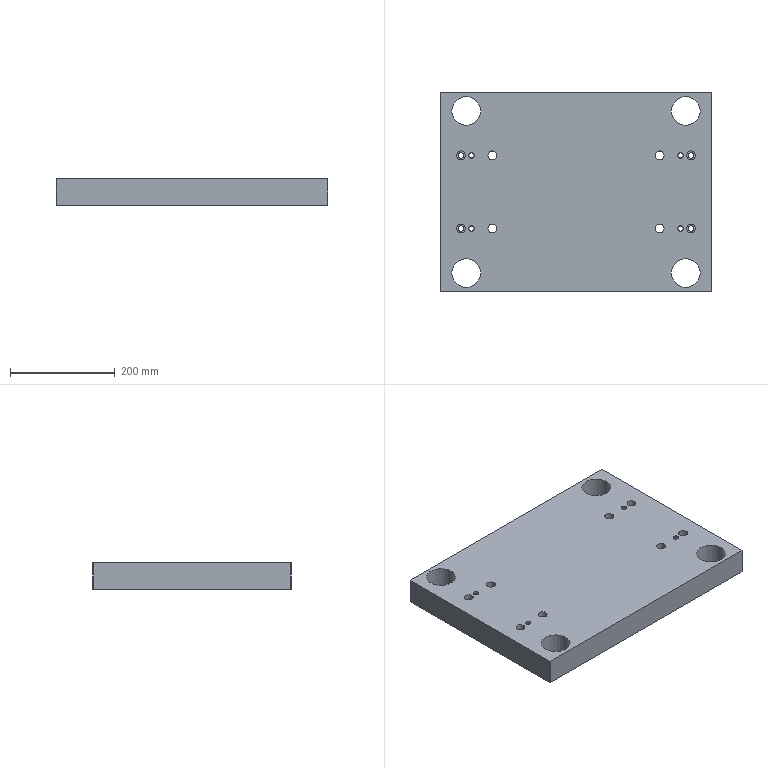Part | NX | features BREP 1 | 1 solid | 42 faces | box 520 x 380 x 50 mm | volume 9317025 mm3 | cylinder 24 | plane 18 | commonest cylinder face diameters 17 x8 10 x4 10.8 x4 11 x4 55 x4
STEP:
#1=CARTESIAN_POINT('',(-260.,-189.,117.));
#2=VERTEX_POINT('',#1);
#3=CARTESIAN_POINT('',(-260.,189.,117.));
#4=VERTEX_POINT('',#3);
#5=CARTESIAN_POINT('',(-260.,-190.,117.));
#6=DIRECTION('',(0.,1.,0.));
#7=VECTOR('',#6,1000.);
#8=LINE('',#5,#7);
#9=EDGE_CURVE('',#2,#4,#8,.T.);
#10=ORIENTED_EDGE('',*,*,#9,.T.);
#11=CARTESIAN_POINT('',(-260.,189.,67.));
#12=VERTEX_POINT('',#11);
#13=CARTESIAN_POINT('',(-260.,189.,67.));
#14=DIRECTION('',(0.,0.,-1.));
#15=VECTOR('',#14,1000.);
#16=LINE('',#13,#15);
#17=EDGE_CURVE('',#4,#12,#16,.T.);
#18=ORIENTED_EDGE('',*,*,#17,.T.);
#19=CARTESIAN_POINT('',(-260.,-189.,67.));
#20=VERTEX_POINT('',#19);
#21=CARTESIAN_POINT('',(-260.,-190.,67.));
#22=DIRECTION('',(0.,1.,0.));
#23=VECTOR('',#22,1000.);
#24=LINE('',#21,#23);
#25=EDGE_CURVE('',#20,#12,#24,.T.);
#26=ORIENTED_EDGE('',*,*,#25,.F.);
#27=CARTESIAN_POINT('',(-260.,-189.,67.));
#28=DIRECTION('',(0.,0.,1.));
#29=VECTOR('',#28,1000.);
#30=LINE('',#27,#29);
#31=EDGE_CURVE('',#20,#2,#30,.T.);
#32=ORIENTED_EDGE('',*,*,#31,.T.);
#33=EDGE_LOOP('',(#10,#18,#26,#32));
#34=FACE_BOUND('',#33,.T.);
#35=CARTESIAN_POINT('',(-260.,-190.,67.));
#36=DIRECTION('',(1.,0.,0.));
#37=DIRECTION('',(0.,0.,1.));
#38=AXIS2_PLACEMENT_3D('',#35,#36,#37);
#39=PLANE('',#38);
#40=ADVANCED_FACE('',(#34),#39,.F.);
#41=CARTESIAN_POINT('',(-259.,190.,67.));
#42=VERTEX_POINT('',#41);
#43=CARTESIAN_POINT('',(259.,190.,67.));
#44=VERTEX_POINT('',#43);
#45=CARTESIAN_POINT('',(-260.,190.,67.));
#46=DIRECTION('',(1.,0.,0.));
#47=VECTOR('',#46,1000.);
#48=LINE('',#45,#47);
#49=EDGE_CURVE('',#42,#44,#48,.T.);
#50=ORIENTED_EDGE('',*,*,#49,.F.);
#51=CARTESIAN_POINT('',(-259.,190.,117.));
#52=VERTEX_POINT('',#51);
#53=CARTESIAN_POINT('',(-259.,190.,67.));
#54=DIRECTION('',(0.,0.,1.));
#55=VECTOR('',#54,1000.);
#56=LINE('',#53,#55);
#57=EDGE_CURVE('',#42,#52,#56,.T.);
#58=ORIENTED_EDGE('',*,*,#57,.T.);
#59=CARTESIAN_POINT('',(259.,190.,117.));
#60=VERTEX_POINT('',#59);
#61=CARTESIAN_POINT('',(-260.,190.,117.));
#62=DIRECTION('',(1.,0.,0.));
#63=VECTOR('',#62,1000.);
#64=LINE('',#61,#63);
#65=EDGE_CURVE('',#52,#60,#64,.T.);
#66=ORIENTED_EDGE('',*,*,#65,.T.);
#67=CARTESIAN_POINT('',(259.,190.,67.));
#68=DIRECTION('',(0.,0.,-1.));
#69=VECTOR('',#68,1000.);
#70=LINE('',#67,#69);
#71=EDGE_CURVE('',#60,#44,#70,.T.);
#72=ORIENTED_EDGE('',*,*,#71,.T.);
#73=EDGE_LOOP('',(#50,#58,#66,#72));
#74=FACE_BOUND('',#73,.T.);
#75=CARTESIAN_POINT('',(-260.,190.,67.));
#76=DIRECTION('',(0.,-1.,0.));
#77=DIRECTION('',(0.,0.,1.));
#78=AXIS2_PLACEMENT_3D('',#75,#76,#77);
#79=PLANE('',#78);
#80=ADVANCED_FACE('',(#74),#79,.F.);
#81=CARTESIAN_POINT('',(260.,189.,67.));
#82=VERTEX_POINT('',#81);
#83=CARTESIAN_POINT('',(260.,-189.,67.));
#84=VERTEX_POINT('',#83);
#85=CARTESIAN_POINT('',(260.,190.,67.));
#86=DIRECTION('',(0.,-1.,0.));
#87=VECTOR('',#86,1000.);
#88=LINE('',#85,#87);
#89=EDGE_CURVE('',#82,#84,#88,.T.);
#90=ORIENTED_EDGE('',*,*,#89,.F.);
#91=CARTESIAN_POINT('',(260.,189.,117.));
#92=VERTEX_POINT('',#91);
#93=CARTESIAN_POINT('',(260.,189.,67.));
#94=DIRECTION('',(0.,0.,1.));
#95=VECTOR('',#94,1000.);
#96=LINE('',#93,#95);
#97=EDGE_CURVE('',#82,#92,#96,.T.);
#98=ORIENTED_EDGE('',*,*,#97,.T.);
#99=CARTESIAN_POINT('',(260.,-189.,117.));
#100=VERTEX_POINT('',#99);
#101=CARTESIAN_POINT('',(260.,190.,117.));
#102=DIRECTION('',(0.,-1.,0.));
#103=VECTOR('',#102,1000.);
#104=LINE('',#101,#103);
#105=EDGE_CURVE('',#92,#100,#104,.T.);
#106=ORIENTED_EDGE('',*,*,#105,.T.);
#107=CARTESIAN_POINT('',(260.,-189.,67.));
#108=DIRECTION('',(0.,0.,-1.));
#109=VECTOR('',#108,1000.);
#110=LINE('',#107,#109);
#111=EDGE_CURVE('',#100,#84,#110,.T.);
#112=ORIENTED_EDGE('',*,*,#111,.T.);
#113=EDGE_LOOP('',(#90,#98,#106,#112));
#114=FACE_BOUND('',#113,.T.);
#115=CARTESIAN_POINT('',(260.,190.,67.));
#116=DIRECTION('',(-1.,0.,0.));
#117=DIRECTION('',(0.,0.,-1.));
#118=AXIS2_PLACEMENT_3D('',#115,#116,#117);
#119=PLANE('',#118);
#120=ADVANCED_FACE('',(#114),#119,.F.);
#121=CARTESIAN_POINT('',(259.,-190.,67.));
#122=VERTEX_POINT('',#121);
#123=CARTESIAN_POINT('',(-259.,-190.,67.));
#124=VERTEX_POINT('',#123);
#125=CARTESIAN_POINT('',(260.,-190.,67.));
#126=DIRECTION('',(-1.,0.,0.));
#127=VECTOR('',#126,1000.);
#128=LINE('',#125,#127);
#129=EDGE_CURVE('',#122,#124,#128,.T.);
#130=ORIENTED_EDGE('',*,*,#129,.F.);
#131=CARTESIAN_POINT('',(259.,-190.,117.));
#132=VERTEX_POINT('',#131);
#133=CARTESIAN_POINT('',(259.,-190.,67.));
#134=DIRECTION('',(0.,0.,1.));
#135=VECTOR('',#134,1000.);
#136=LINE('',#133,#135);
#137=EDGE_CURVE('',#122,#132,#136,.T.);
#138=ORIENTED_EDGE('',*,*,#137,.T.);
#139=CARTESIAN_POINT('',(-259.,-190.,117.));
#140=VERTEX_POINT('',#139);
#141=CARTESIAN_POINT('',(260.,-190.,117.));
#142=DIRECTION('',(-1.,0.,0.));
#143=VECTOR('',#142,1000.);
#144=LINE('',#141,#143);
#145=EDGE_CURVE('',#132,#140,#144,.T.);
#146=ORIENTED_EDGE('',*,*,#145,.T.);
#147=CARTESIAN_POINT('',(-259.,-190.,67.));
#148=DIRECTION('',(0.,0.,-1.));
#149=VECTOR('',#148,1000.);
#150=LINE('',#147,#149);
#151=EDGE_CURVE('',#140,#124,#150,.T.);
#152=ORIENTED_EDGE('',*,*,#151,.T.);
#153=EDGE_LOOP('',(#130,#138,#146,#152));
#154=FACE_BOUND('',#153,.T.);
#155=CARTESIAN_POINT('',(260.,-190.,67.));
#156=DIRECTION('',(0.,1.,0.));
#157=DIRECTION('',(1.,0.,0.));
#158=AXIS2_PLACEMENT_3D('',#155,#156,#157);
#159=PLANE('',#158);
#160=ADVANCED_FACE('',(#154),#159,.F.);
#161=CARTESIAN_POINT('',(182.5,-155.,67.));
#162=VERTEX_POINT('',#161);
#163=CARTESIAN_POINT('',(210.,-155.,67.));
#164=DIRECTION('',(0.,0.,1.));
#165=DIRECTION('',(-1.,0.,0.));
#166=AXIS2_PLACEMENT_3D('',#163,#164,#165);
#167=CIRCLE('',#166,27.5);
#168=EDGE_CURVE('',#162,#162,#167,.T.);
#169=ORIENTED_EDGE('',*,*,#168,.T.);
#170=EDGE_LOOP('',(#169));
#171=FACE_BOUND('',#170,.T.);
#172=CARTESIAN_POINT('',(-237.5,-155.,67.));
#173=VERTEX_POINT('',#172);
#174=CARTESIAN_POINT('',(-210.,-155.,67.));
#175=DIRECTION('',(0.,0.,1.));
#176=DIRECTION('',(-1.,0.,0.));
#177=AXIS2_PLACEMENT_3D('',#174,#175,#176);
#178=CIRCLE('',#177,27.5);
#179=EDGE_CURVE('',#173,#173,#178,.T.);
#180=ORIENTED_EDGE('',*,*,#179,.T.);
#181=EDGE_LOOP('',(#180));
#182=FACE_BOUND('',#181,.T.);
#183=CARTESIAN_POINT('',(-237.5,155.,67.));
#184=VERTEX_POINT('',#183);
#185=CARTESIAN_POINT('',(-210.,155.,67.));
#186=DIRECTION('',(0.,0.,1.));
#187=DIRECTION('',(-1.,0.,0.));
#188=AXIS2_PLACEMENT_3D('',#185,#186,#187);
#189=CIRCLE('',#188,27.5);
#190=EDGE_CURVE('',#184,#184,#189,.T.);
#191=ORIENTED_EDGE('',*,*,#190,.T.);
#192=EDGE_LOOP('',(#191));
#193=FACE_BOUND('',#192,.T.);
#194=CARTESIAN_POINT('',(182.5,155.,67.));
#195=VERTEX_POINT('',#194);
#196=CARTESIAN_POINT('',(210.,155.,67.));
#197=DIRECTION('',(0.,0.,1.));
#198=DIRECTION('',(-1.,0.,0.));
#199=AXIS2_PLACEMENT_3D('',#196,#197,#198);
#200=CIRCLE('',#199,27.5);
#201=EDGE_CURVE('',#195,#195,#200,.T.);
#202=ORIENTED_EDGE('',*,*,#201,.T.);
#203=EDGE_LOOP('',(#202));
#204=FACE_BOUND('',#203,.T.);
#205=CARTESIAN_POINT('',(214.5,-70.,67.));
#206=VERTEX_POINT('',#205);
#207=CARTESIAN_POINT('',(220.,-70.,67.));
#208=DIRECTION('',(0.,0.,-1.));
#209=DIRECTION('',(-1.,0.,0.));
#210=AXIS2_PLACEMENT_3D('',#207,#208,#209);
#211=CIRCLE('',#210,5.5);
#212=EDGE_CURVE('',#206,#206,#211,.T.);
#213=ORIENTED_EDGE('',*,*,#212,.F.);
#214=EDGE_LOOP('',(#213));
#215=FACE_BOUND('',#214,.T.);
#216=CARTESIAN_POINT('',(-225.5,70.,67.));
#217=VERTEX_POINT('',#216);
#218=CARTESIAN_POINT('',(-220.,70.,67.));
#219=DIRECTION('',(0.,0.,-1.));
#220=DIRECTION('',(-1.,0.,0.));
#221=AXIS2_PLACEMENT_3D('',#218,#219,#220);
#222=CIRCLE('',#221,5.5);
#223=EDGE_CURVE('',#217,#217,#222,.T.);
#224=ORIENTED_EDGE('',*,*,#223,.F.);
#225=EDGE_LOOP('',(#224));
#226=FACE_BOUND('',#225,.T.);
#227=CARTESIAN_POINT('',(-225.5,-70.,67.));
#228=VERTEX_POINT('',#227);
#229=CARTESIAN_POINT('',(-220.,-70.,67.));
#230=DIRECTION('',(0.,0.,-1.));
#231=DIRECTION('',(-1.,0.,0.));
#232=AXIS2_PLACEMENT_3D('',#229,#230,#231);
#233=CIRCLE('',#232,5.5);
#234=EDGE_CURVE('',#228,#228,#233,.T.);
#235=ORIENTED_EDGE('',*,*,#234,.F.);
#236=EDGE_LOOP('',(#235));
#237=FACE_BOUND('',#236,.T.);
#238=CARTESIAN_POINT('',(214.5,70.,67.));
#239=VERTEX_POINT('',#238);
#240=CARTESIAN_POINT('',(220.,70.,67.));
#241=DIRECTION('',(0.,0.,-1.));
#242=DIRECTION('',(-1.,0.,0.));
#243=AXIS2_PLACEMENT_3D('',#240,#241,#242);
#244=CIRCLE('',#243,5.5);
#245=EDGE_CURVE('',#239,#239,#244,.T.);
#246=ORIENTED_EDGE('',*,*,#245,.F.);
#247=EDGE_LOOP('',(#246));
#248=FACE_BOUND('',#247,.T.);
#249=CARTESIAN_POINT('',(168.5,-70.,67.));
#250=VERTEX_POINT('',#249);
#251=CARTESIAN_POINT('',(160.,-70.,67.));
#252=DIRECTION('',(0.,0.,1.));
#253=DIRECTION('',(1.,0.,0.));
#254=AXIS2_PLACEMENT_3D('',#251,#252,#253);
#255=CIRCLE('',#254,8.5);
#256=EDGE_CURVE('',#250,#250,#255,.T.);
#257=ORIENTED_EDGE('',*,*,#256,.T.);
#258=EDGE_LOOP('',(#257));
#259=FACE_BOUND('',#258,.T.);
#260=CARTESIAN_POINT('',(-151.5,70.,67.));
#261=VERTEX_POINT('',#260);
#262=CARTESIAN_POINT('',(-160.,70.,67.));
#263=DIRECTION('',(0.,0.,1.));
#264=DIRECTION('',(1.,0.,0.));
#265=AXIS2_PLACEMENT_3D('',#262,#263,#264);
#266=CIRCLE('',#265,8.5);
#267=EDGE_CURVE('',#261,#261,#266,.T.);
#268=ORIENTED_EDGE('',*,*,#267,.T.);
#269=EDGE_LOOP('',(#268));
#270=FACE_BOUND('',#269,.T.);
#271=CARTESIAN_POINT('',(-151.5,-70.,67.));
#272=VERTEX_POINT('',#271);
#273=CARTESIAN_POINT('',(-160.,-70.,67.));
#274=DIRECTION('',(0.,0.,1.));
#275=DIRECTION('',(1.,0.,0.));
#276=AXIS2_PLACEMENT_3D('',#273,#274,#275);
#277=CIRCLE('',#276,8.5);
#278=EDGE_CURVE('',#272,#272,#277,.T.);
#279=ORIENTED_EDGE('',*,*,#278,.T.);
#280=EDGE_LOOP('',(#279));
#281=FACE_BOUND('',#280,.T.);
#282=CARTESIAN_POINT('',(168.5,70.,67.));
#283=VERTEX_POINT('',#282);
#284=CARTESIAN_POINT('',(160.,70.,67.));
#285=DIRECTION('',(0.,0.,1.));
#286=DIRECTION('',(1.,0.,0.));
#287=AXIS2_PLACEMENT_3D('',#284,#285,#286);
#288=CIRCLE('',#287,8.5);
#289=EDGE_CURVE('',#283,#283,#288,.T.);
#290=ORIENTED_EDGE('',*,*,#289,.T.);
#291=EDGE_LOOP('',(#290));
#292=FACE_BOUND('',#291,.T.);
#293=ORIENTED_EDGE('',*,*,#25,.T.);
#294=CARTESIAN_POINT('',(-259.5,189.5,67.));
#295=DIRECTION('',(0.7071,0.7071,0.));
#296=VECTOR('',#295,1000.);
#297=LINE('',#294,#296);
#298=EDGE_CURVE('',#12,#42,#297,.T.);
#299=ORIENTED_EDGE('',*,*,#298,.T.);
#300=ORIENTED_EDGE('',*,*,#49,.T.);
#301=CARTESIAN_POINT('',(-0.5,449.5,67.));
#302=DIRECTION('',(0.7071,-0.7071,0.));
#303=VECTOR('',#302,1000.);
#304=LINE('',#301,#303);
#305=EDGE_CURVE('',#44,#82,#304,.T.);
#306=ORIENTED_EDGE('',*,*,#305,.T.);
#307=ORIENTED_EDGE('',*,*,#89,.T.);
#308=CARTESIAN_POINT('',(189.5,-259.5,67.));
#309=DIRECTION('',(-0.7071,-0.7071,0.));
#310=VECTOR('',#309,1000.);
#311=LINE('',#308,#310);
#312=EDGE_CURVE('',#84,#122,#311,.T.);
#313=ORIENTED_EDGE('',*,*,#312,.T.);
#314=ORIENTED_EDGE('',*,*,#129,.T.);
#315=CARTESIAN_POINT('',(-449.5,0.5,67.));
#316=DIRECTION('',(-0.7071,0.7071,0.));
#317=VECTOR('',#316,1000.);
#318=LINE('',#315,#317);
#319=EDGE_CURVE('',#124,#20,#318,.T.);
#320=ORIENTED_EDGE('',*,*,#319,.T.);
#321=EDGE_LOOP('',(#293,#299,#300,#306,#307,#313,#314,#320));
#322=FACE_BOUND('',#321,.T.);
#323=CARTESIAN_POINT('',(-204.619,-68.085,67.));
#324=VERTEX_POINT('',#323);
#325=CARTESIAN_POINT('',(-200.,-70.,67.));
#326=DIRECTION('',(0.,0.,-1.));
#327=DIRECTION('',(-0.9237,0.383,0.));
#328=AXIS2_PLACEMENT_3D('',#325,#326,#327);
#329=CIRCLE('',#328,5.);
#330=EDGE_CURVE('',#324,#324,#329,.T.);
#331=ORIENTED_EDGE('',*,*,#330,.F.);
#332=EDGE_LOOP('',(#331));
#333=FACE_BOUND('',#332,.T.);
#334=CARTESIAN_POINT('',(-204.619,71.915,67.));
#335=VERTEX_POINT('',#334);
#336=CARTESIAN_POINT('',(-200.,70.,67.));
#337=DIRECTION('',(0.,0.,-1.));
#338=DIRECTION('',(-0.9237,0.383,0.));
#339=AXIS2_PLACEMENT_3D('',#336,#337,#338);
#340=CIRCLE('',#339,5.);
#341=EDGE_CURVE('',#335,#335,#340,.T.);
#342=ORIENTED_EDGE('',*,*,#341,.F.);
#343=EDGE_LOOP('',(#342));
#344=FACE_BOUND('',#343,.T.);
#345=CARTESIAN_POINT('',(195.381,-68.085,67.));
#346=VERTEX_POINT('',#345);
#347=CARTESIAN_POINT('',(200.,-70.,67.));
#348=DIRECTION('',(0.,0.,-1.));
#349=DIRECTION('',(-0.9237,0.383,0.));
#350=AXIS2_PLACEMENT_3D('',#347,#348,#349);
#351=CIRCLE('',#350,5.);
#352=EDGE_CURVE('',#346,#346,#351,.T.);
#353=ORIENTED_EDGE('',*,*,#352,.F.);
#354=EDGE_LOOP('',(#353));
#355=FACE_BOUND('',#354,.T.);
#356=CARTESIAN_POINT('',(195.381,71.915,67.));
#357=VERTEX_POINT('',#356);
#358=CARTESIAN_POINT('',(200.,70.,67.));
#359=DIRECTION('',(0.,0.,-1.));
#360=DIRECTION('',(-0.9237,0.383,0.));
#361=AXIS2_PLACEMENT_3D('',#358,#359,#360);
#362=CIRCLE('',#361,5.);
#363=EDGE_CURVE('',#357,#357,#362,.T.);
#364=ORIENTED_EDGE('',*,*,#363,.F.);
#365=EDGE_LOOP('',(#364));
#366=FACE_BOUND('',#365,.T.);
#367=CARTESIAN_POINT('',(-260.,190.,67.));
#368=DIRECTION('',(0.,0.,-1.));
#369=DIRECTION('',(1.,0.,0.));
#370=AXIS2_PLACEMENT_3D('',#367,#368,#369);
#371=PLANE('',#370);
#372=ADVANCED_FACE('',(#171,#182,#193,#204,#215,#226,#237,#248,#259,#270,#281,#292,#322,#333,#344,#355,#366),#371,.T.);
#373=CARTESIAN_POINT('',(182.5,-155.,117.));
#374=VERTEX_POINT('',#373);
#375=CARTESIAN_POINT('',(210.,-155.,117.));
#376=DIRECTION('',(0.,0.,1.));
#377=DIRECTION('',(-1.,0.,0.));
#378=AXIS2_PLACEMENT_3D('',#375,#376,#377);
#379=CIRCLE('',#378,27.5);
#380=EDGE_CURVE('',#374,#374,#379,.T.);
#381=ORIENTED_EDGE('',*,*,#380,.F.);
#382=EDGE_LOOP('',(#381));
#383=FACE_BOUND('',#382,.T.);
#384=CARTESIAN_POINT('',(-237.5,-155.,117.));
#385=VERTEX_POINT('',#384);
#386=CARTESIAN_POINT('',(-210.,-155.,117.));
#387=DIRECTION('',(0.,0.,1.));
#388=DIRECTION('',(-1.,0.,0.));
#389=AXIS2_PLACEMENT_3D('',#386,#387,#388);
#390=CIRCLE('',#389,27.5);
#391=EDGE_CURVE('',#385,#385,#390,.T.);
#392=ORIENTED_EDGE('',*,*,#391,.F.);
#393=EDGE_LOOP('',(#392));
#394=FACE_BOUND('',#393,.T.);
#395=CARTESIAN_POINT('',(-237.5,155.,117.));
#396=VERTEX_POINT('',#395);
#397=CARTESIAN_POINT('',(-210.,155.,117.));
#398=DIRECTION('',(0.,0.,1.));
#399=DIRECTION('',(-1.,0.,0.));
#400=AXIS2_PLACEMENT_3D('',#397,#398,#399);
#401=CIRCLE('',#400,27.5);
#402=EDGE_CURVE('',#396,#396,#401,.T.);
#403=ORIENTED_EDGE('',*,*,#402,.F.);
#404=EDGE_LOOP('',(#403));
#405=FACE_BOUND('',#404,.T.);
#406=CARTESIAN_POINT('',(182.5,155.,117.));
#407=VERTEX_POINT('',#406);
#408=CARTESIAN_POINT('',(210.,155.,117.));
#409=DIRECTION('',(0.,0.,1.));
#410=DIRECTION('',(-1.,0.,0.));
#411=AXIS2_PLACEMENT_3D('',#408,#409,#410);
#412=CIRCLE('',#411,27.5);
#413=EDGE_CURVE('',#407,#407,#412,.T.);
#414=ORIENTED_EDGE('',*,*,#413,.F.);
#415=EDGE_LOOP('',(#414));
#416=FACE_BOUND('',#415,.T.);
#417=CARTESIAN_POINT('',(204.988,67.932,117.));
#418=VERTEX_POINT('',#417);
#419=CARTESIAN_POINT('',(200.,70.,117.));
#420=DIRECTION('',(0.,0.,1.));
#421=DIRECTION('',(0.9237,-0.383,0.));
#422=AXIS2_PLACEMENT_3D('',#419,#420,#421);
#423=CIRCLE('',#422,5.4);
#424=EDGE_CURVE('',#418,#418,#423,.T.);
#425=ORIENTED_EDGE('',*,*,#424,.F.);
#426=EDGE_LOOP('',(#425));
#427=FACE_BOUND('',#426,.T.);
#428=CARTESIAN_POINT('',(204.988,-72.068,117.));
#429=VERTEX_POINT('',#428);
#430=CARTESIAN_POINT('',(200.,-70.,117.));
#431=DIRECTION('',(0.,0.,1.));
#432=DIRECTION('',(0.9237,-0.383,0.));
#433=AXIS2_PLACEMENT_3D('',#430,#431,#432);
#434=CIRCLE('',#433,5.4);
#435=EDGE_CURVE('',#429,#429,#434,.T.);
#436=ORIENTED_EDGE('',*,*,#435,.F.);
#437=EDGE_LOOP('',(#436));
#438=FACE_BOUND('',#437,.T.);
#439=CARTESIAN_POINT('',(-195.012,67.932,117.));
#440=VERTEX_POINT('',#439);
#441=CARTESIAN_POINT('',(-200.,70.,117.));
#442=DIRECTION('',(0.,0.,1.));
#443=DIRECTION('',(0.9237,-0.383,0.));
#444=AXIS2_PLACEMENT_3D('',#441,#442,#443);
#445=CIRCLE('',#444,5.4);
#446=EDGE_CURVE('',#440,#440,#445,.T.);
#447=ORIENTED_EDGE('',*,*,#446,.F.);
#448=EDGE_LOOP('',(#447));
#449=FACE_BOUND('',#448,.T.);
#450=CARTESIAN_POINT('',(-195.012,-72.068,117.));
#451=VERTEX_POINT('',#450);
#452=CARTESIAN_POINT('',(-200.,-70.,117.));
#453=DIRECTION('',(0.,0.,1.));
#454=DIRECTION('',(0.9237,-0.383,0.));
#455=AXIS2_PLACEMENT_3D('',#452,#453,#454);
#456=CIRCLE('',#455,5.4);
#457=EDGE_CURVE('',#451,#451,#456,.T.);
#458=ORIENTED_EDGE('',*,*,#457,.F.);
#459=EDGE_LOOP('',(#458));
#460=FACE_BOUND('',#459,.T.);
#461=CARTESIAN_POINT('',(228.5,-70.,117.));
#462=VERTEX_POINT('',#461);
#463=CARTESIAN_POINT('',(220.,-70.,117.));
#464=DIRECTION('',(0.,0.,1.));
#465=DIRECTION('',(1.,0.,0.));
#466=AXIS2_PLACEMENT_3D('',#463,#464,#465);
#467=CIRCLE('',#466,8.5);
#468=EDGE_CURVE('',#462,#462,#467,.T.);
#469=ORIENTED_EDGE('',*,*,#468,.F.);
#470=EDGE_LOOP('',(#469));
#471=FACE_BOUND('',#470,.T.);
#472=CARTESIAN_POINT('',(-211.5,70.,117.));
#473=VERTEX_POINT('',#472);
#474=CARTESIAN_POINT('',(-220.,70.,117.));
#475=DIRECTION('',(0.,0.,1.));
#476=DIRECTION('',(1.,0.,0.));
#477=AXIS2_PLACEMENT_3D('',#474,#475,#476);
#478=CIRCLE('',#477,8.5);
#479=EDGE_CURVE('',#473,#473,#478,.T.);
#480=ORIENTED_EDGE('',*,*,#479,.F.);
#481=EDGE_LOOP('',(#480));
#482=FACE_BOUND('',#481,.T.);
#483=CARTESIAN_POINT('',(-211.5,-70.,117.));
#484=VERTEX_POINT('',#483);
#485=CARTESIAN_POINT('',(-220.,-70.,117.));
#486=DIRECTION('',(0.,0.,1.));
#487=DIRECTION('',(1.,0.,0.));
#488=AXIS2_PLACEMENT_3D('',#485,#486,#487);
#489=CIRCLE('',#488,8.5);
#490=EDGE_CURVE('',#484,#484,#489,.T.);
#491=ORIENTED_EDGE('',*,*,#490,.F.);
#492=EDGE_LOOP('',(#491));
#493=FACE_BOUND('',#492,.T.);
#494=CARTESIAN_POINT('',(228.5,70.,117.));
#495=VERTEX_POINT('',#494);
#496=CARTESIAN_POINT('',(220.,70.,117.));
#497=DIRECTION('',(0.,0.,1.));
#498=DIRECTION('',(1.,0.,0.));
#499=AXIS2_PLACEMENT_3D('',#496,#497,#498);
#500=CIRCLE('',#499,8.5);
#501=EDGE_CURVE('',#495,#495,#500,.T.);
#502=ORIENTED_EDGE('',*,*,#501,.F.);
#503=EDGE_LOOP('',(#502));
#504=FACE_BOUND('',#503,.T.);
#505=CARTESIAN_POINT('',(168.5,-70.,117.));
#506=VERTEX_POINT('',#505);
#507=CARTESIAN_POINT('',(160.,-70.,117.));
#508=DIRECTION('',(0.,0.,1.));
#509=DIRECTION('',(1.,0.,0.));
#510=AXIS2_PLACEMENT_3D('',#507,#508,#509);
#511=CIRCLE('',#510,8.5);
#512=EDGE_CURVE('',#506,#506,#511,.T.);
#513=ORIENTED_EDGE('',*,*,#512,.F.);
#514=EDGE_LOOP('',(#513));
#515=FACE_BOUND('',#514,.T.);
#516=CARTESIAN_POINT('',(-151.5,70.,117.));
#517=VERTEX_POINT('',#516);
#518=CARTESIAN_POINT('',(-160.,70.,117.));
#519=DIRECTION('',(0.,0.,1.));
#520=DIRECTION('',(1.,0.,0.));
#521=AXIS2_PLACEMENT_3D('',#518,#519,#520);
#522=CIRCLE('',#521,8.5);
#523=EDGE_CURVE('',#517,#517,#522,.T.);
#524=ORIENTED_EDGE('',*,*,#523,.F.);
#525=EDGE_LOOP('',(#524));
#526=FACE_BOUND('',#525,.T.);
#527=CARTESIAN_POINT('',(-151.5,-70.,117.));
#528=VERTEX_POINT('',#527);
#529=CARTESIAN_POINT('',(-160.,-70.,117.));
#530=DIRECTION('',(0.,0.,1.));
#531=DIRECTION('',(1.,0.,0.));
#532=AXIS2_PLACEMENT_3D('',#529,#530,#531);
#533=CIRCLE('',#532,8.5);
#534=EDGE_CURVE('',#528,#528,#533,.T.);
#535=ORIENTED_EDGE('',*,*,#534,.F.);
#536=EDGE_LOOP('',(#535));
#537=FACE_BOUND('',#536,.T.);
#538=CARTESIAN_POINT('',(168.5,70.,117.));
#539=VERTEX_POINT('',#538);
#540=CARTESIAN_POINT('',(160.,70.,117.));
#541=DIRECTION('',(0.,0.,1.));
#542=DIRECTION('',(1.,0.,0.));
#543=AXIS2_PLACEMENT_3D('',#540,#541,#542);
#544=CIRCLE('',#543,8.5);
#545=EDGE_CURVE('',#539,#539,#544,.T.);
#546=ORIENTED_EDGE('',*,*,#545,.F.);
#547=EDGE_LOOP('',(#546));
#548=FACE_BOUND('',#547,.T.);
#549=ORIENTED_EDGE('',*,*,#65,.F.);
#550=CARTESIAN_POINT('',(-259.,190.,117.));
#551=DIRECTION('',(-0.7071,-0.7071,0.));
#552=VECTOR('',#551,1000.);
#553=LINE('',#550,#552);
#554=EDGE_CURVE('',#52,#4,#553,.T.);
#555=ORIENTED_EDGE('',*,*,#554,.T.);
#556=ORIENTED_EDGE('',*,*,#9,.F.);
#557=CARTESIAN_POINT('',(-260.,-189.,117.));
#558=DIRECTION('',(0.7071,-0.7071,0.));
#559=VECTOR('',#558,1000.);
#560=LINE('',#557,#559);
#561=EDGE_CURVE('',#2,#140,#560,.T.);
#562=ORIENTED_EDGE('',*,*,#561,.T.);
#563=ORIENTED_EDGE('',*,*,#145,.F.);
#564=CARTESIAN_POINT('',(259.,-190.,117.));
#565=DIRECTION('',(0.7071,0.7071,0.));
#566=VECTOR('',#565,1000.);
#567=LINE('',#564,#566);
#568=EDGE_CURVE('',#132,#100,#567,.T.);
#569=ORIENTED_EDGE('',*,*,#568,.T.);
#570=ORIENTED_EDGE('',*,*,#105,.F.);
#571=CARTESIAN_POINT('',(260.,189.,117.));
#572=DIRECTION('',(-0.7071,0.7071,0.));
#573=VECTOR('',#572,1000.);
#574=LINE('',#571,#573);
#575=EDGE_CURVE('',#92,#60,#574,.T.);
#576=ORIENTED_EDGE('',*,*,#575,.T.);
#577=EDGE_LOOP('',(#549,#555,#556,#562,#563,#569,#570,#576));
#578=FACE_BOUND('',#577,.T.);
#579=CARTESIAN_POINT('',(-260.,190.,117.));
#580=DIRECTION('',(0.,0.,-1.));
#581=DIRECTION('',(1.,0.,0.));
#582=AXIS2_PLACEMENT_3D('',#579,#580,#581);
#583=PLANE('',#582);
#584=ADVANCED_FACE('',(#383,#394,#405,#416,#427,#438,#449,#460,#471,#482,#493,#504,#515,#526,#537,#548,#578),#583,.F.);
#585=ORIENTED_EDGE('',*,*,#298,.F.);
#586=ORIENTED_EDGE('',*,*,#17,.F.);
#587=ORIENTED_EDGE('',*,*,#554,.F.);
#588=ORIENTED_EDGE('',*,*,#57,.F.);
#589=EDGE_LOOP('',(#585,#586,#587,#588));
#590=FACE_BOUND('',#589,.T.);
#591=CARTESIAN_POINT('',(-259.,190.,67.));
#592=DIRECTION('',(0.7071,-0.7071,0.));
#593=DIRECTION('',(-0.7071,-0.7071,0.));
#594=AXIS2_PLACEMENT_3D('',#591,#592,#593);
#595=PLANE('',#594);
#596=ADVANCED_FACE('',(#590),#595,.F.);
#597=ORIENTED_EDGE('',*,*,#305,.F.);
#598=ORIENTED_EDGE('',*,*,#71,.F.);
#599=ORIENTED_EDGE('',*,*,#575,.F.);
#600=ORIENTED_EDGE('',*,*,#97,.F.);
#601=EDGE_LOOP('',(#597,#598,#599,#600));
#602=FACE_BOUND('',#601,.T.);
#603=CARTESIAN_POINT('',(260.,189.,67.));
#604=DIRECTION('',(-0.7071,-0.7071,0.));
#605=DIRECTION('',(-0.7071,0.7071,0.));
#606=AXIS2_PLACEMENT_3D('',#603,#604,#605);
#607=PLANE('',#606);
#608=ADVANCED_FACE('',(#602),#607,.F.);
#609=ORIENTED_EDGE('',*,*,#312,.F.);
#610=ORIENTED_EDGE('',*,*,#111,.F.);
#611=ORIENTED_EDGE('',*,*,#568,.F.);
#612=ORIENTED_EDGE('',*,*,#137,.F.);
#613=EDGE_LOOP('',(#609,#610,#611,#612));
#614=FACE_BOUND('',#613,.T.);
#615=CARTESIAN_POINT('',(259.,-190.,67.));
#616=DIRECTION('',(-0.7071,0.7071,0.));
#617=DIRECTION('',(0.7071,0.7071,0.));
#618=AXIS2_PLACEMENT_3D('',#615,#616,#617);
#619=PLANE('',#618);
#620=ADVANCED_FACE('',(#614),#619,.F.);
#621=ORIENTED_EDGE('',*,*,#319,.F.);
#622=ORIENTED_EDGE('',*,*,#151,.F.);
#623=ORIENTED_EDGE('',*,*,#561,.F.);
#624=ORIENTED_EDGE('',*,*,#31,.F.);
#625=EDGE_LOOP('',(#621,#622,#623,#624));
#626=FACE_BOUND('',#625,.T.);
#627=CARTESIAN_POINT('',(-260.,-189.,67.));
#628=DIRECTION('',(0.7071,0.7071,0.));
#629=DIRECTION('',(0.7071,-0.7071,0.));
#630=AXIS2_PLACEMENT_3D('',#627,#628,#629);
#631=PLANE('',#630);
#632=ADVANCED_FACE('',(#626),#631,.F.);
#633=ORIENTED_EDGE('',*,*,#545,.T.);
#634=EDGE_LOOP('',(#633));
#635=FACE_BOUND('',#634,.T.);
#636=ORIENTED_EDGE('',*,*,#289,.F.);
#637=EDGE_LOOP('',(#636));
#638=FACE_BOUND('',#637,.T.);
#639=CARTESIAN_POINT('',(160.,70.,117.));
#640=DIRECTION('',(0.,0.,-1.));
#641=DIRECTION('',(1.,0.,0.));
#642=AXIS2_PLACEMENT_3D('',#639,#640,#641);
#643=CYLINDRICAL_SURFACE('',#642,8.5);
#644=ADVANCED_FACE('',(#635,#638),#643,.F.);
#645=ORIENTED_EDGE('',*,*,#534,.T.);
#646=EDGE_LOOP('',(#645));
#647=FACE_BOUND('',#646,.T.);
#648=ORIENTED_EDGE('',*,*,#278,.F.);
#649=EDGE_LOOP('',(#648));
#650=FACE_BOUND('',#649,.T.);
#651=CARTESIAN_POINT('',(-160.,-70.,117.));
#652=DIRECTION('',(0.,0.,-1.));
#653=DIRECTION('',(1.,0.,0.));
#654=AXIS2_PLACEMENT_3D('',#651,#652,#653);
#655=CYLINDRICAL_SURFACE('',#654,8.5);
#656=ADVANCED_FACE('',(#647,#650),#655,.F.);
#657=ORIENTED_EDGE('',*,*,#523,.T.);
#658=EDGE_LOOP('',(#657));
#659=FACE_BOUND('',#658,.T.);
#660=ORIENTED_EDGE('',*,*,#267,.F.);
#661=EDGE_LOOP('',(#660));
#662=FACE_BOUND('',#661,.T.);
#663=CARTESIAN_POINT('',(-160.,70.,117.));
#664=DIRECTION('',(0.,0.,-1.));
#665=DIRECTION('',(1.,0.,0.));
#666=AXIS2_PLACEMENT_3D('',#663,#664,#665);
#667=CYLINDRICAL_SURFACE('',#666,8.5);
#668=ADVANCED_FACE('',(#659,#662),#667,.F.);
#669=ORIENTED_EDGE('',*,*,#512,.T.);
#670=EDGE_LOOP('',(#669));
#671=FACE_BOUND('',#670,.T.);
#672=ORIENTED_EDGE('',*,*,#256,.F.);
#673=EDGE_LOOP('',(#672));
#674=FACE_BOUND('',#673,.T.);
#675=CARTESIAN_POINT('',(160.,-70.,117.));
#676=DIRECTION('',(0.,0.,-1.));
#677=DIRECTION('',(1.,0.,0.));
#678=AXIS2_PLACEMENT_3D('',#675,#676,#677);
#679=CYLINDRICAL_SURFACE('',#678,8.5);
#680=ADVANCED_FACE('',(#671,#674),#679,.F.);
#681=ORIENTED_EDGE('',*,*,#245,.T.);
#682=EDGE_LOOP('',(#681));
#683=FACE_BOUND('',#682,.T.);
#684=CARTESIAN_POINT('',(214.5,70.,103.));
#685=VERTEX_POINT('',#684);
#686=CARTESIAN_POINT('',(220.,70.,103.));
#687=DIRECTION('',(0.,0.,1.));
#688=DIRECTION('',(-1.,0.,0.));
#689=AXIS2_PLACEMENT_3D('',#686,#687,#688);
#690=CIRCLE('',#689,5.5);
#691=EDGE_CURVE('',#685,#685,#690,.T.);
#692=ORIENTED_EDGE('',*,*,#691,.T.);
#693=EDGE_LOOP('',(#692));
#694=FACE_BOUND('',#693,.T.);
#695=CARTESIAN_POINT('',(220.,70.,103.));
#696=DIRECTION('',(0.,0.,-1.));
#697=DIRECTION('',(1.,0.,0.));
#698=AXIS2_PLACEMENT_3D('',#695,#696,#697);
#699=CYLINDRICAL_SURFACE('',#698,5.5);
#700=ADVANCED_FACE('',(#683,#694),#699,.F.);
#701=ORIENTED_EDGE('',*,*,#501,.T.);
#702=EDGE_LOOP('',(#701));
#703=FACE_BOUND('',#702,.T.);
#704=CARTESIAN_POINT('',(228.5,70.,103.));
#705=VERTEX_POINT('',#704);
#706=CARTESIAN_POINT('',(220.,70.,103.));
#707=DIRECTION('',(0.,0.,-1.));
#708=DIRECTION('',(1.,0.,0.));
#709=AXIS2_PLACEMENT_3D('',#706,#707,#708);
#710=CIRCLE('',#709,8.5);
#711=EDGE_CURVE('',#705,#705,#710,.T.);
#712=ORIENTED_EDGE('',*,*,#711,.T.);
#713=EDGE_LOOP('',(#712));
#714=FACE_BOUND('',#713,.T.);
#715=CARTESIAN_POINT('',(220.,70.,103.));
#716=DIRECTION('',(0.,0.,1.));
#717=DIRECTION('',(-1.,0.,0.));
#718=AXIS2_PLACEMENT_3D('',#715,#716,#717);
#719=CYLINDRICAL_SURFACE('',#718,8.5);
#720=ADVANCED_FACE('',(#703,#714),#719,.F.);
#721=ORIENTED_EDGE('',*,*,#691,.F.);
#722=EDGE_LOOP('',(#721));
#723=FACE_BOUND('',#722,.T.);
#724=ORIENTED_EDGE('',*,*,#711,.F.);
#725=EDGE_LOOP('',(#724));
#726=FACE_BOUND('',#725,.T.);
#727=CARTESIAN_POINT('',(220.,70.,103.));
#728=DIRECTION('',(0.,0.,-1.));
#729=DIRECTION('',(1.,0.,0.));
#730=AXIS2_PLACEMENT_3D('',#727,#728,#729);
#731=PLANE('',#730);
#732=ADVANCED_FACE('',(#723,#726),#731,.F.);
#733=ORIENTED_EDGE('',*,*,#234,.T.);
#734=EDGE_LOOP('',(#733));
#735=FACE_BOUND('',#734,.T.);
#736=CARTESIAN_POINT('',(-225.5,-70.,103.));
#737=VERTEX_POINT('',#736);
#738=CARTESIAN_POINT('',(-220.,-70.,103.));
#739=DIRECTION('',(0.,0.,1.));
#740=DIRECTION('',(-1.,0.,0.));
#741=AXIS2_PLACEMENT_3D('',#738,#739,#740);
#742=CIRCLE('',#741,5.5);
#743=EDGE_CURVE('',#737,#737,#742,.T.);
#744=ORIENTED_EDGE('',*,*,#743,.T.);
#745=EDGE_LOOP('',(#744));
#746=FACE_BOUND('',#745,.T.);
#747=CARTESIAN_POINT('',(-220.,-70.,103.));
#748=DIRECTION('',(0.,0.,-1.));
#749=DIRECTION('',(1.,0.,0.));
#750=AXIS2_PLACEMENT_3D('',#747,#748,#749);
#751=CYLINDRICAL_SURFACE('',#750,5.5);
#752=ADVANCED_FACE('',(#735,#746),#751,.F.);
#753=ORIENTED_EDGE('',*,*,#490,.T.);
#754=EDGE_LOOP('',(#753));
#755=FACE_BOUND('',#754,.T.);
#756=CARTESIAN_POINT('',(-211.5,-70.,103.));
#757=VERTEX_POINT('',#756);
#758=CARTESIAN_POINT('',(-220.,-70.,103.));
#759=DIRECTION('',(0.,0.,-1.));
#760=DIRECTION('',(1.,0.,0.));
#761=AXIS2_PLACEMENT_3D('',#758,#759,#760);
#762=CIRCLE('',#761,8.5);
#763=EDGE_CURVE('',#757,#757,#762,.T.);
#764=ORIENTED_EDGE('',*,*,#763,.T.);
#765=EDGE_LOOP('',(#764));
#766=FACE_BOUND('',#765,.T.);
#767=CARTESIAN_POINT('',(-220.,-70.,103.));
#768=DIRECTION('',(0.,0.,1.));
#769=DIRECTION('',(-1.,0.,0.));
#770=AXIS2_PLACEMENT_3D('',#767,#768,#769);
#771=CYLINDRICAL_SURFACE('',#770,8.5);
#772=ADVANCED_FACE('',(#755,#766),#771,.F.);
#773=ORIENTED_EDGE('',*,*,#743,.F.);
#774=EDGE_LOOP('',(#773));
#775=FACE_BOUND('',#774,.T.);
#776=ORIENTED_EDGE('',*,*,#763,.F.);
#777=EDGE_LOOP('',(#776));
#778=FACE_BOUND('',#777,.T.);
#779=CARTESIAN_POINT('',(-220.,-70.,103.));
#780=DIRECTION('',(0.,0.,-1.));
#781=DIRECTION('',(1.,0.,0.));
#782=AXIS2_PLACEMENT_3D('',#779,#780,#781);
#783=PLANE('',#782);
#784=ADVANCED_FACE('',(#775,#778),#783,.F.);
#785=ORIENTED_EDGE('',*,*,#223,.T.);
#786=EDGE_LOOP('',(#785));
#787=FACE_BOUND('',#786,.T.);
#788=CARTESIAN_POINT('',(-225.5,70.,103.));
#789=VERTEX_POINT('',#788);
#790=CARTESIAN_POINT('',(-220.,70.,103.));
#791=DIRECTION('',(0.,0.,1.));
#792=DIRECTION('',(-1.,0.,0.));
#793=AXIS2_PLACEMENT_3D('',#790,#791,#792);
#794=CIRCLE('',#793,5.5);
#795=EDGE_CURVE('',#789,#789,#794,.T.);
#796=ORIENTED_EDGE('',*,*,#795,.T.);
#797=EDGE_LOOP('',(#796));
#798=FACE_BOUND('',#797,.T.);
#799=CARTESIAN_POINT('',(-220.,70.,103.));
#800=DIRECTION('',(0.,0.,-1.));
#801=DIRECTION('',(1.,0.,0.));
#802=AXIS2_PLACEMENT_3D('',#799,#800,#801);
#803=CYLINDRICAL_SURFACE('',#802,5.5);
#804=ADVANCED_FACE('',(#787,#798),#803,.F.);
#805=ORIENTED_EDGE('',*,*,#479,.T.);
#806=EDGE_LOOP('',(#805));
#807=FACE_BOUND('',#806,.T.);
#808=CARTESIAN_POINT('',(-211.5,70.,103.));
#809=VERTEX_POINT('',#808);
#810=CARTESIAN_POINT('',(-220.,70.,103.));
#811=DIRECTION('',(0.,0.,-1.));
#812=DIRECTION('',(1.,0.,0.));
#813=AXIS2_PLACEMENT_3D('',#810,#811,#812);
#814=CIRCLE('',#813,8.5);
#815=EDGE_CURVE('',#809,#809,#814,.T.);
#816=ORIENTED_EDGE('',*,*,#815,.T.);
#817=EDGE_LOOP('',(#816));
#818=FACE_BOUND('',#817,.T.);
#819=CARTESIAN_POINT('',(-220.,70.,103.));
#820=DIRECTION('',(0.,0.,1.));
#821=DIRECTION('',(-1.,0.,0.));
#822=AXIS2_PLACEMENT_3D('',#819,#820,#821);
#823=CYLINDRICAL_SURFACE('',#822,8.5);
#824=ADVANCED_FACE('',(#807,#818),#823,.F.);
#825=ORIENTED_EDGE('',*,*,#795,.F.);
#826=EDGE_LOOP('',(#825));
#827=FACE_BOUND('',#826,.T.);
#828=ORIENTED_EDGE('',*,*,#815,.F.);
#829=EDGE_LOOP('',(#828));
#830=FACE_BOUND('',#829,.T.);
#831=CARTESIAN_POINT('',(-220.,70.,103.));
#832=DIRECTION('',(0.,0.,-1.));
#833=DIRECTION('',(1.,0.,0.));
#834=AXIS2_PLACEMENT_3D('',#831,#832,#833);
#835=PLANE('',#834);
#836=ADVANCED_FACE('',(#827,#830),#835,.F.);
#837=ORIENTED_EDGE('',*,*,#212,.T.);
#838=EDGE_LOOP('',(#837));
#839=FACE_BOUND('',#838,.T.);
#840=CARTESIAN_POINT('',(214.5,-70.,103.));
#841=VERTEX_POINT('',#840);
#842=CARTESIAN_POINT('',(220.,-70.,103.));
#843=DIRECTION('',(0.,0.,1.));
#844=DIRECTION('',(-1.,0.,0.));
#845=AXIS2_PLACEMENT_3D('',#842,#843,#844);
#846=CIRCLE('',#845,5.5);
#847=EDGE_CURVE('',#841,#841,#846,.T.);
#848=ORIENTED_EDGE('',*,*,#847,.T.);
#849=EDGE_LOOP('',(#848));
#850=FACE_BOUND('',#849,.T.);
#851=CARTESIAN_POINT('',(220.,-70.,103.));
#852=DIRECTION('',(0.,0.,-1.));
#853=DIRECTION('',(1.,0.,0.));
#854=AXIS2_PLACEMENT_3D('',#851,#852,#853);
#855=CYLINDRICAL_SURFACE('',#854,5.5);
#856=ADVANCED_FACE('',(#839,#850),#855,.F.);
#857=ORIENTED_EDGE('',*,*,#468,.T.);
#858=EDGE_LOOP('',(#857));
#859=FACE_BOUND('',#858,.T.);
#860=CARTESIAN_POINT('',(228.5,-70.,103.));
#861=VERTEX_POINT('',#860);
#862=CARTESIAN_POINT('',(220.,-70.,103.));
#863=DIRECTION('',(0.,0.,-1.));
#864=DIRECTION('',(1.,0.,0.));
#865=AXIS2_PLACEMENT_3D('',#862,#863,#864);
#866=CIRCLE('',#865,8.5);
#867=EDGE_CURVE('',#861,#861,#866,.T.);
#868=ORIENTED_EDGE('',*,*,#867,.T.);
#869=EDGE_LOOP('',(#868));
#870=FACE_BOUND('',#869,.T.);
#871=CARTESIAN_POINT('',(220.,-70.,103.));
#872=DIRECTION('',(0.,0.,1.));
#873=DIRECTION('',(-1.,0.,0.));
#874=AXIS2_PLACEMENT_3D('',#871,#872,#873);
#875=CYLINDRICAL_SURFACE('',#874,8.5);
#876=ADVANCED_FACE('',(#859,#870),#875,.F.);
#877=ORIENTED_EDGE('',*,*,#847,.F.);
#878=EDGE_LOOP('',(#877));
#879=FACE_BOUND('',#878,.T.);
#880=ORIENTED_EDGE('',*,*,#867,.F.);
#881=EDGE_LOOP('',(#880));
#882=FACE_BOUND('',#881,.T.);
#883=CARTESIAN_POINT('',(220.,-70.,103.));
#884=DIRECTION('',(0.,0.,-1.));
#885=DIRECTION('',(1.,0.,0.));
#886=AXIS2_PLACEMENT_3D('',#883,#884,#885);
#887=PLANE('',#886);
#888=ADVANCED_FACE('',(#879,#882),#887,.F.);
#889=CARTESIAN_POINT('',(-195.012,-72.068,113.));
#890=VERTEX_POINT('',#889);
#891=CARTESIAN_POINT('',(-200.,-70.,113.));
#892=DIRECTION('',(0.,0.,-1.));
#893=DIRECTION('',(0.9237,-0.383,0.));
#894=AXIS2_PLACEMENT_3D('',#891,#892,#893);
#895=CIRCLE('',#894,5.4);
#896=EDGE_CURVE('',#890,#890,#895,.T.);
#897=ORIENTED_EDGE('',*,*,#896,.T.);
#898=EDGE_LOOP('',(#897));
#899=FACE_BOUND('',#898,.T.);
#900=ORIENTED_EDGE('',*,*,#457,.T.);
#901=EDGE_LOOP('',(#900));
#902=FACE_BOUND('',#901,.T.);
#903=CARTESIAN_POINT('',(-200.,-70.,113.));
#904=DIRECTION('',(0.,0.,1.));
#905=DIRECTION('',(-0.9237,0.383,0.));
#906=AXIS2_PLACEMENT_3D('',#903,#904,#905);
#907=CYLINDRICAL_SURFACE('',#906,5.4);
#908=ADVANCED_FACE('',(#899,#902),#907,.F.);
#909=CARTESIAN_POINT('',(-204.619,-68.085,113.));
#910=VERTEX_POINT('',#909);
#911=CARTESIAN_POINT('',(-200.,-70.,113.));
#912=DIRECTION('',(0.,0.,1.));
#913=DIRECTION('',(-0.9237,0.383,0.));
#914=AXIS2_PLACEMENT_3D('',#911,#912,#913);
#915=CIRCLE('',#914,5.);
#916=EDGE_CURVE('',#910,#910,#915,.T.);
#917=ORIENTED_EDGE('',*,*,#916,.F.);
#918=EDGE_LOOP('',(#917));
#919=FACE_BOUND('',#918,.T.);
#920=ORIENTED_EDGE('',*,*,#896,.F.);
#921=EDGE_LOOP('',(#920));
#922=FACE_BOUND('',#921,.T.);
#923=CARTESIAN_POINT('',(-200.,-70.,113.));
#924=DIRECTION('',(0.,0.,1.));
#925=DIRECTION('',(-0.9237,0.383,0.));
#926=AXIS2_PLACEMENT_3D('',#923,#924,#925);
#927=PLANE('',#926);
#928=ADVANCED_FACE('',(#919,#922),#927,.T.);
#929=ORIENTED_EDGE('',*,*,#330,.T.);
#930=EDGE_LOOP('',(#929));
#931=FACE_BOUND('',#930,.T.);
#932=ORIENTED_EDGE('',*,*,#916,.T.);
#933=EDGE_LOOP('',(#932));
#934=FACE_BOUND('',#933,.T.);
#935=CARTESIAN_POINT('',(-200.,-70.,113.));
#936=DIRECTION('',(0.,0.,-1.));
#937=DIRECTION('',(0.9237,-0.383,0.));
#938=AXIS2_PLACEMENT_3D('',#935,#936,#937);
#939=CYLINDRICAL_SURFACE('',#938,5.);
#940=ADVANCED_FACE('',(#931,#934),#939,.F.);
#941=CARTESIAN_POINT('',(-195.012,67.932,113.));
#942=VERTEX_POINT('',#941);
#943=CARTESIAN_POINT('',(-200.,70.,113.));
#944=DIRECTION('',(0.,0.,-1.));
#945=DIRECTION('',(0.9237,-0.383,0.));
#946=AXIS2_PLACEMENT_3D('',#943,#944,#945);
#947=CIRCLE('',#946,5.4);
#948=EDGE_CURVE('',#942,#942,#947,.T.);
#949=ORIENTED_EDGE('',*,*,#948,.T.);
#950=EDGE_LOOP('',(#949));
#951=FACE_BOUND('',#950,.T.);
#952=ORIENTED_EDGE('',*,*,#446,.T.);
#953=EDGE_LOOP('',(#952));
#954=FACE_BOUND('',#953,.T.);
#955=CARTESIAN_POINT('',(-200.,70.,113.));
#956=DIRECTION('',(0.,0.,1.));
#957=DIRECTION('',(-0.9237,0.383,0.));
#958=AXIS2_PLACEMENT_3D('',#955,#956,#957);
#959=CYLINDRICAL_SURFACE('',#958,5.4);
#960=ADVANCED_FACE('',(#951,#954),#959,.F.);
#961=CARTESIAN_POINT('',(-204.619,71.915,113.));
#962=VERTEX_POINT('',#961);
#963=CARTESIAN_POINT('',(-200.,70.,113.));
#964=DIRECTION('',(0.,0.,1.));
#965=DIRECTION('',(-0.9237,0.383,0.));
#966=AXIS2_PLACEMENT_3D('',#963,#964,#965);
#967=CIRCLE('',#966,5.);
#968=EDGE_CURVE('',#962,#962,#967,.T.);
#969=ORIENTED_EDGE('',*,*,#968,.F.);
#970=EDGE_LOOP('',(#969));
#971=FACE_BOUND('',#970,.T.);
#972=ORIENTED_EDGE('',*,*,#948,.F.);
#973=EDGE_LOOP('',(#972));
#974=FACE_BOUND('',#973,.T.);
#975=CARTESIAN_POINT('',(-200.,70.,113.));
#976=DIRECTION('',(0.,0.,1.));
#977=DIRECTION('',(-0.9237,0.383,0.));
#978=AXIS2_PLACEMENT_3D('',#975,#976,#977);
#979=PLANE('',#978);
#980=ADVANCED_FACE('',(#971,#974),#979,.T.);
#981=ORIENTED_EDGE('',*,*,#341,.T.);
#982=EDGE_LOOP('',(#981));
#983=FACE_BOUND('',#982,.T.);
#984=ORIENTED_EDGE('',*,*,#968,.T.);
#985=EDGE_LOOP('',(#984));
#986=FACE_BOUND('',#985,.T.);
#987=CARTESIAN_POINT('',(-200.,70.,113.));
#988=DIRECTION('',(0.,0.,-1.));
#989=DIRECTION('',(0.9237,-0.383,0.));
#990=AXIS2_PLACEMENT_3D('',#987,#988,#989);
#991=CYLINDRICAL_SURFACE('',#990,5.);
#992=ADVANCED_FACE('',(#983,#986),#991,.F.);
#993=CARTESIAN_POINT('',(204.988,-72.068,113.));
#994=VERTEX_POINT('',#993);
#995=CARTESIAN_POINT('',(200.,-70.,113.));
#996=DIRECTION('',(0.,0.,-1.));
#997=DIRECTION('',(0.9237,-0.383,0.));
#998=AXIS2_PLACEMENT_3D('',#995,#996,#997);
#999=CIRCLE('',#998,5.4);
#1000=EDGE_CURVE('',#994,#994,#999,.T.);
#1001=ORIENTED_EDGE('',*,*,#1000,.T.);
#1002=EDGE_LOOP('',(#1001));
#1003=FACE_BOUND('',#1002,.T.);
#1004=ORIENTED_EDGE('',*,*,#435,.T.);
#1005=EDGE_LOOP('',(#1004));
#1006=FACE_BOUND('',#1005,.T.);
#1007=CARTESIAN_POINT('',(200.,-70.,113.));
#1008=DIRECTION('',(0.,0.,1.));
#1009=DIRECTION('',(-0.9237,0.383,0.));
#1010=AXIS2_PLACEMENT_3D('',#1007,#1008,#1009);
#1011=CYLINDRICAL_SURFACE('',#1010,5.4);
#1012=ADVANCED_FACE('',(#1003,#1006),#1011,.F.);
#1013=CARTESIAN_POINT('',(195.381,-68.085,113.));
#1014=VERTEX_POINT('',#1013);
#1015=CARTESIAN_POINT('',(200.,-70.,113.));
#1016=DIRECTION('',(0.,0.,1.));
#1017=DIRECTION('',(-0.9237,0.383,0.));
#1018=AXIS2_PLACEMENT_3D('',#1015,#1016,#1017);
#1019=CIRCLE('',#1018,5.);
#1020=EDGE_CURVE('',#1014,#1014,#1019,.T.);
#1021=ORIENTED_EDGE('',*,*,#1020,.F.);
#1022=EDGE_LOOP('',(#1021));
#1023=FACE_BOUND('',#1022,.T.);
#1024=ORIENTED_EDGE('',*,*,#1000,.F.);
#1025=EDGE_LOOP('',(#1024));
#1026=FACE_BOUND('',#1025,.T.);
#1027=CARTESIAN_POINT('',(200.,-70.,113.));
#1028=DIRECTION('',(0.,0.,1.));
#1029=DIRECTION('',(-0.9237,0.383,0.));
#1030=AXIS2_PLACEMENT_3D('',#1027,#1028,#1029);
#1031=PLANE('',#1030);
#1032=ADVANCED_FACE('',(#1023,#1026),#1031,.T.);
#1033=ORIENTED_EDGE('',*,*,#352,.T.);
#1034=EDGE_LOOP('',(#1033));
#1035=FACE_BOUND('',#1034,.T.);
#1036=ORIENTED_EDGE('',*,*,#1020,.T.);
#1037=EDGE_LOOP('',(#1036));
#1038=FACE_BOUND('',#1037,.T.);
#1039=CARTESIAN_POINT('',(200.,-70.,113.));
#1040=DIRECTION('',(0.,0.,-1.));
#1041=DIRECTION('',(0.9237,-0.383,0.));
#1042=AXIS2_PLACEMENT_3D('',#1039,#1040,#1041);
#1043=CYLINDRICAL_SURFACE('',#1042,5.);
#1044=ADVANCED_FACE('',(#1035,#1038),#1043,.F.);
#1045=CARTESIAN_POINT('',(204.988,67.932,113.));
#1046=VERTEX_POINT('',#1045);
#1047=CARTESIAN_POINT('',(200.,70.,113.));
#1048=DIRECTION('',(0.,0.,-1.));
#1049=DIRECTION('',(0.9237,-0.383,0.));
#1050=AXIS2_PLACEMENT_3D('',#1047,#1048,#1049);
#1051=CIRCLE('',#1050,5.4);
#1052=EDGE_CURVE('',#1046,#1046,#1051,.T.);
#1053=ORIENTED_EDGE('',*,*,#1052,.T.);
#1054=EDGE_LOOP('',(#1053));
#1055=FACE_BOUND('',#1054,.T.);
#1056=ORIENTED_EDGE('',*,*,#424,.T.);
#1057=EDGE_LOOP('',(#1056));
#1058=FACE_BOUND('',#1057,.T.);
#1059=CARTESIAN_POINT('',(200.,70.,113.));
#1060=DIRECTION('',(0.,0.,1.));
#1061=DIRECTION('',(-0.9237,0.383,0.));
#1062=AXIS2_PLACEMENT_3D('',#1059,#1060,#1061);
#1063=CYLINDRICAL_SURFACE('',#1062,5.4);
#1064=ADVANCED_FACE('',(#1055,#1058),#1063,.F.);
#1065=CARTESIAN_POINT('',(195.381,71.915,113.));
#1066=VERTEX_POINT('',#1065);
#1067=CARTESIAN_POINT('',(200.,70.,113.));
#1068=DIRECTION('',(0.,0.,1.));
#1069=DIRECTION('',(-0.9237,0.383,0.));
#1070=AXIS2_PLACEMENT_3D('',#1067,#1068,#1069);
#1071=CIRCLE('',#1070,5.);
#1072=EDGE_CURVE('',#1066,#1066,#1071,.T.);
#1073=ORIENTED_EDGE('',*,*,#1072,.F.);
#1074=EDGE_LOOP('',(#1073));
#1075=FACE_BOUND('',#1074,.T.);
#1076=ORIENTED_EDGE('',*,*,#1052,.F.);
#1077=EDGE_LOOP('',(#1076));
#1078=FACE_BOUND('',#1077,.T.);
#1079=CARTESIAN_POINT('',(200.,70.,113.));
#1080=DIRECTION('',(0.,0.,1.));
#1081=DIRECTION('',(-0.9237,0.383,0.));
#1082=AXIS2_PLACEMENT_3D('',#1079,#1080,#1081);
#1083=PLANE('',#1082);
#1084=ADVANCED_FACE('',(#1075,#1078),#1083,.T.);
#1085=ORIENTED_EDGE('',*,*,#363,.T.);
#1086=EDGE_LOOP('',(#1085));
#1087=FACE_BOUND('',#1086,.T.);
#1088=ORIENTED_EDGE('',*,*,#1072,.T.);
#1089=EDGE_LOOP('',(#1088));
#1090=FACE_BOUND('',#1089,.T.);
#1091=CARTESIAN_POINT('',(200.,70.,113.));
#1092=DIRECTION('',(0.,0.,-1.));
#1093=DIRECTION('',(0.9237,-0.383,0.));
#1094=AXIS2_PLACEMENT_3D('',#1091,#1092,#1093);
#1095=CYLINDRICAL_SURFACE('',#1094,5.);
#1096=ADVANCED_FACE('',(#1087,#1090),#1095,.F.);
#1097=ORIENTED_EDGE('',*,*,#201,.F.);
#1098=EDGE_LOOP('',(#1097));
#1099=FACE_BOUND('',#1098,.T.);
#1100=ORIENTED_EDGE('',*,*,#413,.T.);
#1101=EDGE_LOOP('',(#1100));
#1102=FACE_BOUND('',#1101,.T.);
#1103=CARTESIAN_POINT('',(210.,155.,118.4));
#1104=DIRECTION('',(0.,0.,-1.));
#1105=DIRECTION('',(1.,0.,0.));
#1106=AXIS2_PLACEMENT_3D('',#1103,#1104,#1105);
#1107=CYLINDRICAL_SURFACE('',#1106,27.5);
#1108=ADVANCED_FACE('',(#1099,#1102),#1107,.F.);
#1109=ORIENTED_EDGE('',*,*,#190,.F.);
#1110=EDGE_LOOP('',(#1109));
#1111=FACE_BOUND('',#1110,.T.);
#1112=ORIENTED_EDGE('',*,*,#402,.T.);
#1113=EDGE_LOOP('',(#1112));
#1114=FACE_BOUND('',#1113,.T.);
#1115=CARTESIAN_POINT('',(-210.,155.,118.4));
#1116=DIRECTION('',(0.,0.,-1.));
#1117=DIRECTION('',(1.,0.,0.));
#1118=AXIS2_PLACEMENT_3D('',#1115,#1116,#1117);
#1119=CYLINDRICAL_SURFACE('',#1118,27.5);
#1120=ADVANCED_FACE('',(#1111,#1114),#1119,.F.);
#1121=ORIENTED_EDGE('',*,*,#179,.F.);
#1122=EDGE_LOOP('',(#1121));
#1123=FACE_BOUND('',#1122,.T.);
#1124=ORIENTED_EDGE('',*,*,#391,.T.);
#1125=EDGE_LOOP('',(#1124));
#1126=FACE_BOUND('',#1125,.T.);
#1127=CARTESIAN_POINT('',(-210.,-155.,118.4));
#1128=DIRECTION('',(0.,0.,-1.));
#1129=DIRECTION('',(1.,0.,0.));
#1130=AXIS2_PLACEMENT_3D('',#1127,#1128,#1129);
#1131=CYLINDRICAL_SURFACE('',#1130,27.5);
#1132=ADVANCED_FACE('',(#1123,#1126),#1131,.F.);
#1133=ORIENTED_EDGE('',*,*,#168,.F.);
#1134=EDGE_LOOP('',(#1133));
#1135=FACE_BOUND('',#1134,.T.);
#1136=ORIENTED_EDGE('',*,*,#380,.T.);
#1137=EDGE_LOOP('',(#1136));
#1138=FACE_BOUND('',#1137,.T.);
#1139=CARTESIAN_POINT('',(210.,-155.,118.4));
#1140=DIRECTION('',(0.,0.,-1.));
#1141=DIRECTION('',(1.,0.,0.));
#1142=AXIS2_PLACEMENT_3D('',#1139,#1140,#1141);
#1143=CYLINDRICAL_SURFACE('',#1142,27.5);
#1144=ADVANCED_FACE('',(#1135,#1138),#1143,.F.);
#1145=CLOSED_SHELL('',(#40,#80,#120,#160,#372,#584,#596,#608,#620,#632,#644,#656,#668,#680,#700,#720,#732,#752,#772,#784,#804,#824,#836,#856,#876,#888,#908,#928,#940,#960,#980,#992,#1012,#1032,#1044,#1064,#1084,#1096,#1108,#1120,#1132,#1144));
#1146=MANIFOLD_SOLID_BREP('',#1145);
#1147=(LENGTH_UNIT()NAMED_UNIT(*)SI_UNIT(.MILLI.,.METRE.));
#1148=UNCERTAINTY_MEASURE_WITH_UNIT(LENGTH_MEASURE(0.00001),#1147,'','');
#1149=(NAMED_UNIT(*)PLANE_ANGLE_UNIT()SI_UNIT($,.RADIAN.));
#1150=(NAMED_UNIT(*)SI_UNIT($,.STERADIAN.)SOLID_ANGLE_UNIT());
#1151=(GEOMETRIC_REPRESENTATION_CONTEXT(3)GLOBAL_UNCERTAINTY_ASSIGNED_CONTEXT((#1148))GLOBAL_UNIT_ASSIGNED_CONTEXT((#1147,#1149,#1150))REPRESENTATION_CONTEXT('',''));
#1152=ADVANCED_BREP_SHAPE_REPRESENTATION('',(#1146),#1151);